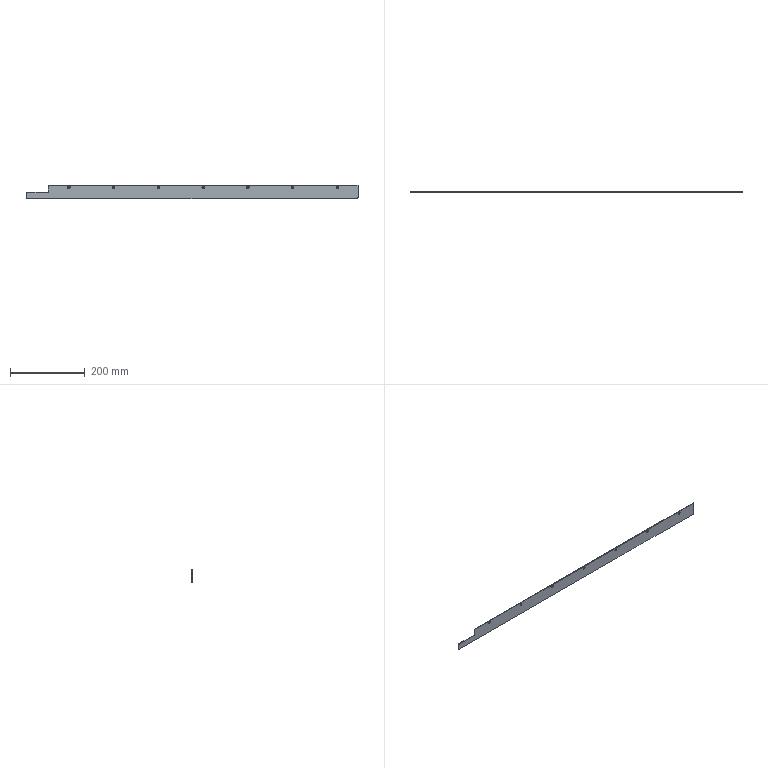Part | STEP file | BZJ-BZMM-JDKTBDYY Product限位Plate一 | 1 solid | 39 faces | box 890 x 2 x 35 mm | volume 59822 mm3 | cylinder 17 | cone 14 | plane 8 | commonest cylinder face diameters 3.4 x14 4 x3